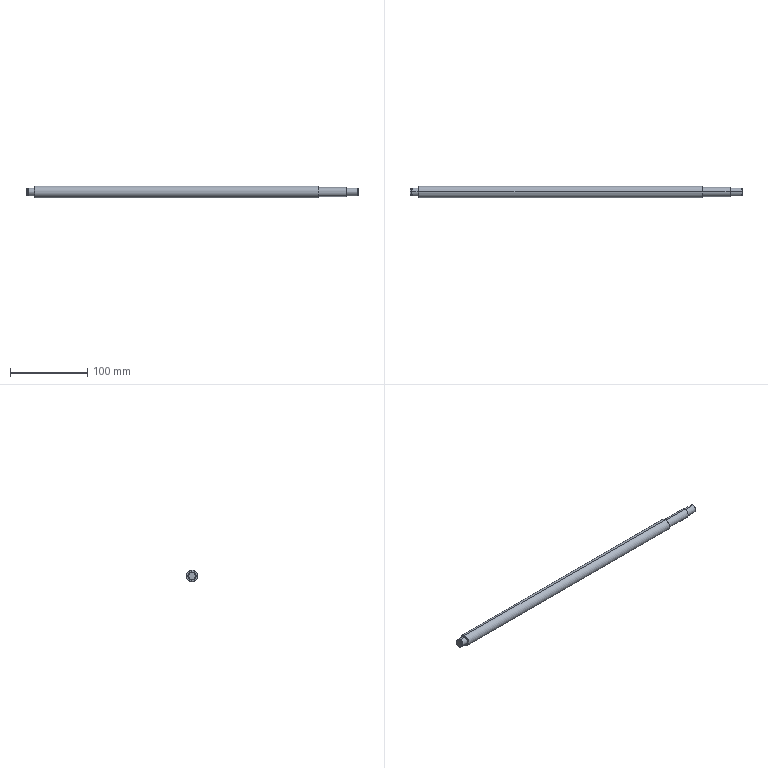Part | SolidWorks | features Revolution 8, RevCut 7, ICE 5, RefAxis 3, Fillet 2 | 1 solid | 35 faces | box 430 x 15 x 15 mm | volume 71115 mm3 | cylinder 12 | cone 10 | plane 7 | torus 6 | commonest cylinder face diameters 10 x6 9.6 x2 12 x2 15 x2
STEP:
#1=CARTESIAN_POINT('',(430.,0.,4.5));
#2=VERTEX_POINT('',#1);
#3=CARTESIAN_POINT('',(430.,0.,-4.5));
#4=VERTEX_POINT('',#3);
#5=CARTESIAN_POINT('',(430.,0.,0.));
#6=DIRECTION('',(-1.,0.,0.));
#7=DIRECTION('',(0.,0.,1.));
#8=AXIS2_PLACEMENT_3D('',#5,#6,#7);
#9=CIRCLE('',#8,4.5);
#10=EDGE_CURVE('',#2,#4,#9,.T.);
#11=ORIENTED_EDGE('',*,*,#10,.T.);
#12=CARTESIAN_POINT('',(429.5,0.,-5.));
#13=VERTEX_POINT('',#12);
#14=CARTESIAN_POINT('',(430.,0.,-4.5));
#15=DIRECTION('',(-0.7071,0.,-0.7071));
#16=VECTOR('',#15,1000.);
#17=LINE('',#14,#16);
#18=EDGE_CURVE('',#4,#13,#17,.T.);
#19=ORIENTED_EDGE('',*,*,#18,.T.);
#20=CARTESIAN_POINT('',(429.5,0.,5.));
#21=VERTEX_POINT('',#20);
#22=CARTESIAN_POINT('',(429.5,0.,0.));
#23=DIRECTION('',(-1.,0.,0.));
#24=DIRECTION('',(0.,0.,1.));
#25=AXIS2_PLACEMENT_3D('',#22,#23,#24);
#26=CIRCLE('',#25,5.);
#27=EDGE_CURVE('',#21,#13,#26,.T.);
#28=ORIENTED_EDGE('',*,*,#27,.F.);
#29=CARTESIAN_POINT('',(430.,0.,4.5));
#30=DIRECTION('',(-0.7071,0.,0.7071));
#31=VECTOR('',#30,1000.);
#32=LINE('',#29,#31);
#33=EDGE_CURVE('',#2,#21,#32,.T.);
#34=ORIENTED_EDGE('',*,*,#33,.F.);
#35=EDGE_LOOP('',(#11,#19,#28,#34));
#36=FACE_OUTER_BOUND('',#35,.T.);
#37=CARTESIAN_POINT('',(430.,0.,0.));
#38=DIRECTION('',(-1.,0.,0.));
#39=DIRECTION('',(0.,0.,1.));
#40=AXIS2_PLACEMENT_3D('',#37,#38,#39);
#41=CONICAL_SURFACE('',#40,4.5,0.7854);
#42=ADVANCED_FACE('',(#36),#41,.T.);
#43=ORIENTED_EDGE('',*,*,#27,.T.);
#44=CARTESIAN_POINT('',(415.2,0.,-5.));
#45=VERTEX_POINT('',#44);
#46=CARTESIAN_POINT('',(-7.5,0.,-5.));
#47=DIRECTION('',(-1.,0.,0.));
#48=VECTOR('',#47,1000.);
#49=LINE('',#46,#48);
#50=EDGE_CURVE('',#13,#45,#49,.T.);
#51=ORIENTED_EDGE('',*,*,#50,.T.);
#52=CARTESIAN_POINT('',(415.2,0.,5.));
#53=VERTEX_POINT('',#52);
#54=CARTESIAN_POINT('',(415.2,0.,0.));
#55=DIRECTION('',(-1.,0.,0.));
#56=DIRECTION('',(0.,0.,1.));
#57=AXIS2_PLACEMENT_3D('',#54,#55,#56);
#58=CIRCLE('',#57,5.);
#59=EDGE_CURVE('',#53,#45,#58,.T.);
#60=ORIENTED_EDGE('',*,*,#59,.F.);
#61=CARTESIAN_POINT('',(-7.5,0.,5.));
#62=DIRECTION('',(-1.,0.,0.));
#63=VECTOR('',#62,1000.);
#64=LINE('',#61,#63);
#65=EDGE_CURVE('',#21,#53,#64,.T.);
#66=ORIENTED_EDGE('',*,*,#65,.F.);
#67=EDGE_LOOP('',(#43,#51,#60,#66));
#68=FACE_OUTER_BOUND('',#67,.T.);
#69=CARTESIAN_POINT('',(-7.5,0.,0.));
#70=DIRECTION('',(-1.,0.,0.));
#71=DIRECTION('',(0.,0.,1.));
#72=AXIS2_PLACEMENT_3D('',#69,#70,#71);
#73=CYLINDRICAL_SURFACE('',#72,5.);
#74=ADVANCED_FACE('',(#68),#73,.T.);
#75=CARTESIAN_POINT('',(415.,0.,-5.2));
#76=VERTEX_POINT('',#75);
#77=CARTESIAN_POINT('',(415.,0.,5.2));
#78=VERTEX_POINT('',#77);
#79=CARTESIAN_POINT('',(415.,0.,0.));
#80=DIRECTION('',(-1.,0.,0.));
#81=DIRECTION('',(0.,0.,1.));
#82=AXIS2_PLACEMENT_3D('',#79,#80,#81);
#83=CIRCLE('',#82,5.2);
#84=EDGE_CURVE('',#76,#78,#83,.T.);
#85=ORIENTED_EDGE('',*,*,#84,.F.);
#86=CARTESIAN_POINT('',(415.2,0.,-5.2));
#87=DIRECTION('',(0.,1.,0.));
#88=DIRECTION('',(0.,0.,1.));
#89=AXIS2_PLACEMENT_3D('',#86,#87,#88);
#90=CIRCLE('',#89,0.2);
#91=EDGE_CURVE('',#76,#45,#90,.T.);
#92=ORIENTED_EDGE('',*,*,#91,.T.);
#93=CARTESIAN_POINT('',(415.2,0.,0.));
#94=DIRECTION('',(-1.,0.,0.));
#95=DIRECTION('',(0.,0.,1.));
#96=AXIS2_PLACEMENT_3D('',#93,#94,#95);
#97=CIRCLE('',#96,5.);
#98=EDGE_CURVE('',#45,#53,#97,.T.);
#99=ORIENTED_EDGE('',*,*,#98,.T.);
#100=CARTESIAN_POINT('',(415.2,0.,5.2));
#101=DIRECTION('',(0.,-1.,0.));
#102=DIRECTION('',(0.,0.,-1.));
#103=AXIS2_PLACEMENT_3D('',#100,#101,#102);
#104=CIRCLE('',#103,0.2);
#105=EDGE_CURVE('',#78,#53,#104,.T.);
#106=ORIENTED_EDGE('',*,*,#105,.F.);
#107=EDGE_LOOP('',(#85,#92,#99,#106));
#108=FACE_OUTER_BOUND('',#107,.T.);
#109=CARTESIAN_POINT('',(415.2,0.,0.));
#110=DIRECTION('',(-1.,0.,0.));
#111=DIRECTION('',(0.,0.,1.));
#112=AXIS2_PLACEMENT_3D('',#109,#110,#111);
#113=TOROIDAL_SURFACE('',#112,5.2,0.2);
#114=ADVANCED_FACE('',(#108),#113,.F.);
#115=CARTESIAN_POINT('',(415.,0.,5.5));
#116=VERTEX_POINT('',#115);
#117=CARTESIAN_POINT('',(415.,0.,-5.5));
#118=VERTEX_POINT('',#117);
#119=CARTESIAN_POINT('',(415.,0.,0.));
#120=DIRECTION('',(-1.,0.,0.));
#121=DIRECTION('',(0.,0.,1.));
#122=AXIS2_PLACEMENT_3D('',#119,#120,#121);
#123=CIRCLE('',#122,5.5);
#124=EDGE_CURVE('',#116,#118,#123,.T.);
#125=ORIENTED_EDGE('',*,*,#124,.T.);
#126=CARTESIAN_POINT('',(414.5,0.,-6.));
#127=VERTEX_POINT('',#126);
#128=CARTESIAN_POINT('',(415.,0.,-5.5));
#129=DIRECTION('',(-0.7071,0.,-0.7071));
#130=VECTOR('',#129,1000.);
#131=LINE('',#128,#130);
#132=EDGE_CURVE('',#118,#127,#131,.T.);
#133=ORIENTED_EDGE('',*,*,#132,.T.);
#134=CARTESIAN_POINT('',(414.5,0.,6.));
#135=VERTEX_POINT('',#134);
#136=CARTESIAN_POINT('',(414.5,0.,0.));
#137=DIRECTION('',(-1.,0.,0.));
#138=DIRECTION('',(0.,0.,1.));
#139=AXIS2_PLACEMENT_3D('',#136,#137,#138);
#140=CIRCLE('',#139,6.);
#141=EDGE_CURVE('',#135,#127,#140,.T.);
#142=ORIENTED_EDGE('',*,*,#141,.F.);
#143=CARTESIAN_POINT('',(415.,0.,5.5));
#144=DIRECTION('',(-0.7071,0.,0.7071));
#145=VECTOR('',#144,1000.);
#146=LINE('',#143,#145);
#147=EDGE_CURVE('',#116,#135,#146,.T.);
#148=ORIENTED_EDGE('',*,*,#147,.F.);
#149=EDGE_LOOP('',(#125,#133,#142,#148));
#150=FACE_OUTER_BOUND('',#149,.T.);
#151=CARTESIAN_POINT('',(415.,0.,0.));
#152=DIRECTION('',(-1.,0.,0.));
#153=DIRECTION('',(0.,0.,1.));
#154=AXIS2_PLACEMENT_3D('',#151,#152,#153);
#155=CONICAL_SURFACE('',#154,5.5,0.7854);
#156=ADVANCED_FACE('',(#150),#155,.T.);
#157=ORIENTED_EDGE('',*,*,#141,.T.);
#158=CARTESIAN_POINT('',(379.3,0.,-6.));
#159=VERTEX_POINT('',#158);
#160=CARTESIAN_POINT('',(-7.5,0.,-6.));
#161=DIRECTION('',(-1.,0.,0.));
#162=VECTOR('',#161,1000.);
#163=LINE('',#160,#162);
#164=EDGE_CURVE('',#127,#159,#163,.T.);
#165=ORIENTED_EDGE('',*,*,#164,.T.);
#166=CARTESIAN_POINT('',(379.3,0.,6.));
#167=VERTEX_POINT('',#166);
#168=CARTESIAN_POINT('',(379.3,0.,0.));
#169=DIRECTION('',(-1.,0.,0.));
#170=DIRECTION('',(0.,0.,1.));
#171=AXIS2_PLACEMENT_3D('',#168,#169,#170);
#172=CIRCLE('',#171,6.);
#173=EDGE_CURVE('',#167,#159,#172,.T.);
#174=ORIENTED_EDGE('',*,*,#173,.F.);
#175=CARTESIAN_POINT('',(-7.5,0.,6.));
#176=DIRECTION('',(-1.,0.,0.));
#177=VECTOR('',#176,1000.);
#178=LINE('',#175,#177);
#179=EDGE_CURVE('',#135,#167,#178,.T.);
#180=ORIENTED_EDGE('',*,*,#179,.F.);
#181=EDGE_LOOP('',(#157,#165,#174,#180));
#182=FACE_OUTER_BOUND('',#181,.T.);
#183=CARTESIAN_POINT('',(-7.5,0.,0.));
#184=DIRECTION('',(-1.,0.,0.));
#185=DIRECTION('',(0.,0.,1.));
#186=AXIS2_PLACEMENT_3D('',#183,#184,#185);
#187=CYLINDRICAL_SURFACE('',#186,6.);
#188=ADVANCED_FACE('',(#182),#187,.T.);
#189=CARTESIAN_POINT('',(379.,0.,-6.3));
#190=VERTEX_POINT('',#189);
#191=CARTESIAN_POINT('',(379.,0.,6.3));
#192=VERTEX_POINT('',#191);
#193=CARTESIAN_POINT('',(379.,0.,0.));
#194=DIRECTION('',(-1.,0.,0.));
#195=DIRECTION('',(0.,0.,1.));
#196=AXIS2_PLACEMENT_3D('',#193,#194,#195);
#197=CIRCLE('',#196,6.3);
#198=EDGE_CURVE('',#190,#192,#197,.T.);
#199=ORIENTED_EDGE('',*,*,#198,.F.);
#200=CARTESIAN_POINT('',(379.3,0.,-6.3));
#201=DIRECTION('',(0.,1.,0.));
#202=DIRECTION('',(0.,0.,1.));
#203=AXIS2_PLACEMENT_3D('',#200,#201,#202);
#204=CIRCLE('',#203,0.3);
#205=EDGE_CURVE('',#190,#159,#204,.T.);
#206=ORIENTED_EDGE('',*,*,#205,.T.);
#207=CARTESIAN_POINT('',(379.3,0.,0.));
#208=DIRECTION('',(-1.,0.,0.));
#209=DIRECTION('',(0.,0.,1.));
#210=AXIS2_PLACEMENT_3D('',#207,#208,#209);
#211=CIRCLE('',#210,6.);
#212=EDGE_CURVE('',#159,#167,#211,.T.);
#213=ORIENTED_EDGE('',*,*,#212,.T.);
#214=CARTESIAN_POINT('',(379.3,0.,6.3));
#215=DIRECTION('',(0.,-1.,0.));
#216=DIRECTION('',(0.,0.,-1.));
#217=AXIS2_PLACEMENT_3D('',#214,#215,#216);
#218=CIRCLE('',#217,0.3);
#219=EDGE_CURVE('',#192,#167,#218,.T.);
#220=ORIENTED_EDGE('',*,*,#219,.F.);
#221=EDGE_LOOP('',(#199,#206,#213,#220));
#222=FACE_OUTER_BOUND('',#221,.T.);
#223=CARTESIAN_POINT('',(379.3,0.,0.));
#224=DIRECTION('',(-1.,0.,0.));
#225=DIRECTION('',(0.,0.,1.));
#226=AXIS2_PLACEMENT_3D('',#223,#224,#225);
#227=TOROIDAL_SURFACE('',#226,6.3,0.3);
#228=ADVANCED_FACE('',(#222),#227,.F.);
#229=CARTESIAN_POINT('',(379.,0.,7.));
#230=VERTEX_POINT('',#229);
#231=CARTESIAN_POINT('',(379.,0.,-7.));
#232=VERTEX_POINT('',#231);
#233=CARTESIAN_POINT('',(379.,0.,0.));
#234=DIRECTION('',(-1.,0.,0.));
#235=DIRECTION('',(0.,0.,1.));
#236=AXIS2_PLACEMENT_3D('',#233,#234,#235);
#237=CIRCLE('',#236,7.);
#238=EDGE_CURVE('',#230,#232,#237,.T.);
#239=ORIENTED_EDGE('',*,*,#238,.T.);
#240=CARTESIAN_POINT('',(378.5,0.,-7.5));
#241=VERTEX_POINT('',#240);
#242=CARTESIAN_POINT('',(379.,0.,-7.));
#243=DIRECTION('',(-0.7071,0.,-0.7071));
#244=VECTOR('',#243,1000.);
#245=LINE('',#242,#244);
#246=EDGE_CURVE('',#232,#241,#245,.T.);
#247=ORIENTED_EDGE('',*,*,#246,.T.);
#248=CARTESIAN_POINT('',(378.5,0.,7.5));
#249=VERTEX_POINT('',#248);
#250=CARTESIAN_POINT('',(378.5,0.,0.));
#251=DIRECTION('',(-1.,0.,0.));
#252=DIRECTION('',(0.,0.,1.));
#253=AXIS2_PLACEMENT_3D('',#250,#251,#252);
#254=CIRCLE('',#253,7.5);
#255=EDGE_CURVE('',#249,#241,#254,.T.);
#256=ORIENTED_EDGE('',*,*,#255,.F.);
#257=CARTESIAN_POINT('',(379.,0.,7.));
#258=DIRECTION('',(-0.7071,0.,0.7071));
#259=VECTOR('',#258,1000.);
#260=LINE('',#257,#259);
#261=EDGE_CURVE('',#230,#249,#260,.T.);
#262=ORIENTED_EDGE('',*,*,#261,.F.);
#263=EDGE_LOOP('',(#239,#247,#256,#262));
#264=FACE_OUTER_BOUND('',#263,.T.);
#265=CARTESIAN_POINT('',(379.,0.,0.));
#266=DIRECTION('',(-1.,0.,0.));
#267=DIRECTION('',(0.,0.,1.));
#268=AXIS2_PLACEMENT_3D('',#265,#266,#267);
#269=CONICAL_SURFACE('',#268,7.,0.7854);
#270=ADVANCED_FACE('',(#264),#269,.T.);
#271=ORIENTED_EDGE('',*,*,#255,.T.);
#272=CARTESIAN_POINT('',(11.5,0.,-7.5));
#273=VERTEX_POINT('',#272);
#274=CARTESIAN_POINT('',(-7.5,0.,-7.5));
#275=DIRECTION('',(-1.,0.,0.));
#276=VECTOR('',#275,1000.);
#277=LINE('',#274,#276);
#278=EDGE_CURVE('',#241,#273,#277,.T.);
#279=ORIENTED_EDGE('',*,*,#278,.T.);
#280=CARTESIAN_POINT('',(11.5,0.,7.5));
#281=VERTEX_POINT('',#280);
#282=CARTESIAN_POINT('',(11.5,0.,0.));
#283=DIRECTION('',(-1.,0.,0.));
#284=DIRECTION('',(0.,0.,1.));
#285=AXIS2_PLACEMENT_3D('',#282,#283,#284);
#286=CIRCLE('',#285,7.5);
#287=EDGE_CURVE('',#281,#273,#286,.T.);
#288=ORIENTED_EDGE('',*,*,#287,.F.);
#289=CARTESIAN_POINT('',(-7.5,0.,7.5));
#290=DIRECTION('',(-1.,0.,0.));
#291=VECTOR('',#290,1000.);
#292=LINE('',#289,#291);
#293=EDGE_CURVE('',#249,#281,#292,.T.);
#294=ORIENTED_EDGE('',*,*,#293,.F.);
#295=EDGE_LOOP('',(#271,#279,#288,#294));
#296=FACE_OUTER_BOUND('',#295,.T.);
#297=CARTESIAN_POINT('',(-7.5,0.,0.));
#298=DIRECTION('',(-1.,0.,0.));
#299=DIRECTION('',(0.,0.,1.));
#300=AXIS2_PLACEMENT_3D('',#297,#298,#299);
#301=CYLINDRICAL_SURFACE('',#300,7.5);
#302=ADVANCED_FACE('',(#296),#301,.T.);
#303=CARTESIAN_POINT('',(11.,0.,7.));
#304=VERTEX_POINT('',#303);
#305=CARTESIAN_POINT('',(11.,0.,-7.));
#306=VERTEX_POINT('',#305);
#307=CARTESIAN_POINT('',(11.,0.,0.));
#308=DIRECTION('',(-1.,0.,0.));
#309=DIRECTION('',(0.,0.,1.));
#310=AXIS2_PLACEMENT_3D('',#307,#308,#309);
#311=CIRCLE('',#310,7.);
#312=EDGE_CURVE('',#304,#306,#311,.T.);
#313=ORIENTED_EDGE('',*,*,#312,.F.);
#314=CARTESIAN_POINT('',(11.5,0.,7.5));
#315=DIRECTION('',(0.7071,0.,0.7071));
#316=VECTOR('',#315,1000.);
#317=LINE('',#314,#316);
#318=EDGE_CURVE('',#304,#281,#317,.T.);
#319=ORIENTED_EDGE('',*,*,#318,.T.);
#320=ORIENTED_EDGE('',*,*,#287,.T.);
#321=CARTESIAN_POINT('',(11.5,0.,-7.5));
#322=DIRECTION('',(0.7071,0.,-0.7071));
#323=VECTOR('',#322,1000.);
#324=LINE('',#321,#323);
#325=EDGE_CURVE('',#306,#273,#324,.T.);
#326=ORIENTED_EDGE('',*,*,#325,.F.);
#327=EDGE_LOOP('',(#313,#319,#320,#326));
#328=FACE_OUTER_BOUND('',#327,.T.);
#329=CARTESIAN_POINT('',(11.5,0.,0.));
#330=DIRECTION('',(1.,0.,0.));
#331=DIRECTION('',(0.,0.,-1.));
#332=AXIS2_PLACEMENT_3D('',#329,#330,#331);
#333=CONICAL_SURFACE('',#332,7.5,0.7854);
#334=ADVANCED_FACE('',(#328),#333,.T.);
#335=CARTESIAN_POINT('',(10.7,0.,-5.));
#336=VERTEX_POINT('',#335);
#337=CARTESIAN_POINT('',(10.7,0.,5.));
#338=VERTEX_POINT('',#337);
#339=CARTESIAN_POINT('',(10.7,0.,0.));
#340=DIRECTION('',(-1.,0.,0.));
#341=DIRECTION('',(0.,0.,1.));
#342=AXIS2_PLACEMENT_3D('',#339,#340,#341);
#343=CIRCLE('',#342,5.);
#344=EDGE_CURVE('',#336,#338,#343,.T.);
#345=ORIENTED_EDGE('',*,*,#344,.F.);
#346=CARTESIAN_POINT('',(11.,0.,-5.3));
#347=VERTEX_POINT('',#346);
#348=CARTESIAN_POINT('',(10.7,0.,-5.3));
#349=DIRECTION('',(0.,1.,0.));
#350=DIRECTION('',(0.,0.,1.));
#351=AXIS2_PLACEMENT_3D('',#348,#349,#350);
#352=CIRCLE('',#351,0.3);
#353=EDGE_CURVE('',#336,#347,#352,.T.);
#354=ORIENTED_EDGE('',*,*,#353,.T.);
#355=CARTESIAN_POINT('',(11.,0.,5.3));
#356=VERTEX_POINT('',#355);
#357=CARTESIAN_POINT('',(11.,0.,0.));
#358=DIRECTION('',(-1.,0.,0.));
#359=DIRECTION('',(0.,0.,1.));
#360=AXIS2_PLACEMENT_3D('',#357,#358,#359);
#361=CIRCLE('',#360,5.3);
#362=EDGE_CURVE('',#347,#356,#361,.T.);
#363=ORIENTED_EDGE('',*,*,#362,.T.);
#364=CARTESIAN_POINT('',(10.7,0.,5.3));
#365=DIRECTION('',(0.,-1.,0.));
#366=DIRECTION('',(0.,0.,-1.));
#367=AXIS2_PLACEMENT_3D('',#364,#365,#366);
#368=CIRCLE('',#367,0.3);
#369=EDGE_CURVE('',#338,#356,#368,.T.);
#370=ORIENTED_EDGE('',*,*,#369,.F.);
#371=EDGE_LOOP('',(#345,#354,#363,#370));
#372=FACE_OUTER_BOUND('',#371,.T.);
#373=CARTESIAN_POINT('',(10.7,0.,0.));
#374=DIRECTION('',(-1.,0.,0.));
#375=DIRECTION('',(0.,0.,1.));
#376=AXIS2_PLACEMENT_3D('',#373,#374,#375);
#377=TOROIDAL_SURFACE('',#376,5.3,0.3);
#378=ADVANCED_FACE('',(#372),#377,.F.);
#379=CARTESIAN_POINT('',(10.7,0.,0.));
#380=DIRECTION('',(-1.,0.,0.));
#381=DIRECTION('',(0.,0.,1.));
#382=AXIS2_PLACEMENT_3D('',#379,#380,#381);
#383=CIRCLE('',#382,5.);
#384=EDGE_CURVE('',#338,#336,#383,.T.);
#385=ORIENTED_EDGE('',*,*,#384,.T.);
#386=CARTESIAN_POINT('',(3.,0.,-5.));
#387=VERTEX_POINT('',#386);
#388=CARTESIAN_POINT('',(-7.5,0.,-5.));
#389=DIRECTION('',(-1.,0.,0.));
#390=VECTOR('',#389,1000.);
#391=LINE('',#388,#390);
#392=EDGE_CURVE('',#336,#387,#391,.T.);
#393=ORIENTED_EDGE('',*,*,#392,.T.);
#394=CARTESIAN_POINT('',(3.,0.,5.));
#395=VERTEX_POINT('',#394);
#396=CARTESIAN_POINT('',(3.,0.,0.));
#397=DIRECTION('',(-1.,0.,0.));
#398=DIRECTION('',(0.,0.,1.));
#399=AXIS2_PLACEMENT_3D('',#396,#397,#398);
#400=CIRCLE('',#399,5.);
#401=EDGE_CURVE('',#395,#387,#400,.T.);
#402=ORIENTED_EDGE('',*,*,#401,.F.);
#403=CARTESIAN_POINT('',(-7.5,0.,5.));
#404=DIRECTION('',(-1.,0.,0.));
#405=VECTOR('',#404,1000.);
#406=LINE('',#403,#405);
#407=EDGE_CURVE('',#338,#395,#406,.T.);
#408=ORIENTED_EDGE('',*,*,#407,.F.);
#409=EDGE_LOOP('',(#385,#393,#402,#408));
#410=FACE_OUTER_BOUND('',#409,.T.);
#411=CARTESIAN_POINT('',(-7.5,0.,0.));
#412=DIRECTION('',(-1.,0.,0.));
#413=DIRECTION('',(0.,0.,1.));
#414=AXIS2_PLACEMENT_3D('',#411,#412,#413);
#415=CYLINDRICAL_SURFACE('',#414,5.);
#416=ADVANCED_FACE('',(#410),#415,.T.);
#417=CARTESIAN_POINT('',(3.,0.,4.8));
#418=VERTEX_POINT('',#417);
#419=CARTESIAN_POINT('',(3.,0.,-4.8));
#420=VERTEX_POINT('',#419);
#421=CARTESIAN_POINT('',(3.,0.,0.));
#422=DIRECTION('',(-1.,0.,0.));
#423=DIRECTION('',(0.,0.,1.));
#424=AXIS2_PLACEMENT_3D('',#421,#422,#423);
#425=CIRCLE('',#424,4.8);
#426=EDGE_CURVE('',#418,#420,#425,.T.);
#427=ORIENTED_EDGE('',*,*,#426,.T.);
#428=CARTESIAN_POINT('',(1.85,0.,-4.8));
#429=VERTEX_POINT('',#428);
#430=CARTESIAN_POINT('',(-7.5,0.,-4.8));
#431=DIRECTION('',(-1.,0.,0.));
#432=VECTOR('',#431,1000.);
#433=LINE('',#430,#432);
#434=EDGE_CURVE('',#420,#429,#433,.T.);
#435=ORIENTED_EDGE('',*,*,#434,.T.);
#436=CARTESIAN_POINT('',(1.85,0.,4.8));
#437=VERTEX_POINT('',#436);
#438=CARTESIAN_POINT('',(1.85,0.,0.));
#439=DIRECTION('',(-1.,0.,0.));
#440=DIRECTION('',(0.,0.,1.));
#441=AXIS2_PLACEMENT_3D('',#438,#439,#440);
#442=CIRCLE('',#441,4.8);
#443=EDGE_CURVE('',#437,#429,#442,.T.);
#444=ORIENTED_EDGE('',*,*,#443,.F.);
#445=CARTESIAN_POINT('',(-7.5,0.,4.8));
#446=DIRECTION('',(-1.,0.,0.));
#447=VECTOR('',#446,1000.);
#448=LINE('',#445,#447);
#449=EDGE_CURVE('',#418,#437,#448,.T.);
#450=ORIENTED_EDGE('',*,*,#449,.F.);
#451=EDGE_LOOP('',(#427,#435,#444,#450));
#452=FACE_OUTER_BOUND('',#451,.T.);
#453=CARTESIAN_POINT('',(-7.5,0.,0.));
#454=DIRECTION('',(-1.,0.,0.));
#455=DIRECTION('',(0.,0.,1.));
#456=AXIS2_PLACEMENT_3D('',#453,#454,#455);
#457=CYLINDRICAL_SURFACE('',#456,4.8);
#458=ADVANCED_FACE('',(#452),#457,.T.);
#459=CARTESIAN_POINT('',(1.85,0.,5.));
#460=VERTEX_POINT('',#459);
#461=CARTESIAN_POINT('',(1.85,0.,-5.));
#462=VERTEX_POINT('',#461);
#463=CARTESIAN_POINT('',(1.85,0.,0.));
#464=DIRECTION('',(-1.,0.,0.));
#465=DIRECTION('',(0.,0.,1.));
#466=AXIS2_PLACEMENT_3D('',#463,#464,#465);
#467=CIRCLE('',#466,5.);
#468=EDGE_CURVE('',#460,#462,#467,.T.);
#469=ORIENTED_EDGE('',*,*,#468,.T.);
#470=CARTESIAN_POINT('',(0.5,0.,-5.));
#471=VERTEX_POINT('',#470);
#472=CARTESIAN_POINT('',(-7.5,0.,-5.));
#473=DIRECTION('',(-1.,0.,0.));
#474=VECTOR('',#473,1000.);
#475=LINE('',#472,#474);
#476=EDGE_CURVE('',#462,#471,#475,.T.);
#477=ORIENTED_EDGE('',*,*,#476,.T.);
#478=CARTESIAN_POINT('',(0.5,0.,5.));
#479=VERTEX_POINT('',#478);
#480=CARTESIAN_POINT('',(0.5,0.,0.));
#481=DIRECTION('',(-1.,0.,0.));
#482=DIRECTION('',(0.,0.,1.));
#483=AXIS2_PLACEMENT_3D('',#480,#481,#482);
#484=CIRCLE('',#483,5.);
#485=EDGE_CURVE('',#479,#471,#484,.T.);
#486=ORIENTED_EDGE('',*,*,#485,.F.);
#487=CARTESIAN_POINT('',(-7.5,0.,5.));
#488=DIRECTION('',(-1.,0.,0.));
#489=VECTOR('',#488,1000.);
#490=LINE('',#487,#489);
#491=EDGE_CURVE('',#460,#479,#490,.T.);
#492=ORIENTED_EDGE('',*,*,#491,.F.);
#493=EDGE_LOOP('',(#469,#477,#486,#492));
#494=FACE_OUTER_BOUND('',#493,.T.);
#495=CARTESIAN_POINT('',(-7.5,0.,0.));
#496=DIRECTION('',(-1.,0.,0.));
#497=DIRECTION('',(0.,0.,1.));
#498=AXIS2_PLACEMENT_3D('',#495,#496,#497);
#499=CYLINDRICAL_SURFACE('',#498,5.);
#500=ADVANCED_FACE('',(#494),#499,.T.);
#501=CARTESIAN_POINT('',(0.,0.,4.5));
#502=VERTEX_POINT('',#501);
#503=CARTESIAN_POINT('',(0.,0.,-4.5));
#504=VERTEX_POINT('',#503);
#505=CARTESIAN_POINT('',(0.,0.,0.));
#506=DIRECTION('',(-1.,0.,0.));
#507=DIRECTION('',(0.,0.,1.));
#508=AXIS2_PLACEMENT_3D('',#505,#506,#507);
#509=CIRCLE('',#508,4.5);
#510=EDGE_CURVE('',#502,#504,#509,.T.);
#511=ORIENTED_EDGE('',*,*,#510,.F.);
#512=CARTESIAN_POINT('',(0.5,0.,5.));
#513=DIRECTION('',(0.7071,0.,0.7071));
#514=VECTOR('',#513,1000.);
#515=LINE('',#512,#514);
#516=EDGE_CURVE('',#502,#479,#515,.T.);
#517=ORIENTED_EDGE('',*,*,#516,.T.);
#518=ORIENTED_EDGE('',*,*,#485,.T.);
#519=CARTESIAN_POINT('',(0.5,0.,-5.));
#520=DIRECTION('',(0.7071,0.,-0.7071));
#521=VECTOR('',#520,1000.);
#522=LINE('',#519,#521);
#523=EDGE_CURVE('',#504,#471,#522,.T.);
#524=ORIENTED_EDGE('',*,*,#523,.F.);
#525=EDGE_LOOP('',(#511,#517,#518,#524));
#526=FACE_OUTER_BOUND('',#525,.T.);
#527=CARTESIAN_POINT('',(0.5,0.,0.));
#528=DIRECTION('',(1.,0.,0.));
#529=DIRECTION('',(0.,0.,-1.));
#530=AXIS2_PLACEMENT_3D('',#527,#528,#529);
#531=CONICAL_SURFACE('',#530,5.,0.7854);
#532=ADVANCED_FACE('',(#526),#531,.T.);
#533=ORIENTED_EDGE('',*,*,#516,.F.);
#534=CARTESIAN_POINT('',(0.,0.,0.));
#535=DIRECTION('',(-1.,0.,0.));
#536=DIRECTION('',(0.,0.,1.));
#537=AXIS2_PLACEMENT_3D('',#534,#535,#536);
#538=CIRCLE('',#537,4.5);
#539=EDGE_CURVE('',#504,#502,#538,.T.);
#540=ORIENTED_EDGE('',*,*,#539,.F.);
#541=ORIENTED_EDGE('',*,*,#523,.T.);
#542=CARTESIAN_POINT('',(0.5,0.,0.));
#543=DIRECTION('',(-1.,0.,0.));
#544=DIRECTION('',(0.,0.,1.));
#545=AXIS2_PLACEMENT_3D('',#542,#543,#544);
#546=CIRCLE('',#545,5.);
#547=EDGE_CURVE('',#471,#479,#546,.T.);
#548=ORIENTED_EDGE('',*,*,#547,.T.);
#549=EDGE_LOOP('',(#533,#540,#541,#548));
#550=FACE_OUTER_BOUND('',#549,.T.);
#551=CARTESIAN_POINT('',(0.5,0.,0.));
#552=DIRECTION('',(1.,0.,0.));
#553=DIRECTION('',(0.,0.,-1.));
#554=AXIS2_PLACEMENT_3D('',#551,#552,#553);
#555=CONICAL_SURFACE('',#554,5.,0.7854);
#556=ADVANCED_FACE('',(#550),#555,.T.);
#557=ORIENTED_EDGE('',*,*,#476,.F.);
#558=CARTESIAN_POINT('',(1.85,0.,0.));
#559=DIRECTION('',(-1.,0.,0.));
#560=DIRECTION('',(0.,0.,1.));
#561=AXIS2_PLACEMENT_3D('',#558,#559,#560);
#562=CIRCLE('',#561,5.);
#563=EDGE_CURVE('',#462,#460,#562,.T.);
#564=ORIENTED_EDGE('',*,*,#563,.T.);
#565=ORIENTED_EDGE('',*,*,#491,.T.);
#566=ORIENTED_EDGE('',*,*,#547,.F.);
#567=EDGE_LOOP('',(#557,#564,#565,#566));
#568=FACE_OUTER_BOUND('',#567,.T.);
#569=CARTESIAN_POINT('',(-7.5,0.,0.));
#570=DIRECTION('',(-1.,0.,0.));
#571=DIRECTION('',(0.,0.,1.));
#572=AXIS2_PLACEMENT_3D('',#569,#570,#571);
#573=CYLINDRICAL_SURFACE('',#572,5.);
#574=ADVANCED_FACE('',(#568),#573,.T.);
#575=ORIENTED_EDGE('',*,*,#468,.F.);
#576=ORIENTED_EDGE('',*,*,#563,.F.);
#577=EDGE_LOOP('',(#575,#576));
#578=FACE_OUTER_BOUND('',#577,.T.);
#579=ORIENTED_EDGE('',*,*,#443,.T.);
#580=CARTESIAN_POINT('',(1.85,0.,0.));
#581=DIRECTION('',(-1.,0.,0.));
#582=DIRECTION('',(0.,0.,1.));
#583=AXIS2_PLACEMENT_3D('',#580,#581,#582);
#584=CIRCLE('',#583,4.8);
#585=EDGE_CURVE('',#429,#437,#584,.T.);
#586=ORIENTED_EDGE('',*,*,#585,.T.);
#587=EDGE_LOOP('',(#579,#586));
#588=FACE_BOUND('',#587,.T.);
#589=CARTESIAN_POINT('',(1.85,5.,0.));
#590=DIRECTION('',(-1.,0.,0.));
#591=DIRECTION('',(0.,0.,1.));
#592=AXIS2_PLACEMENT_3D('',#589,#590,#591);
#593=PLANE('',#592);
#594=ADVANCED_FACE('',(#578,#588),#593,.F.);
#595=ORIENTED_EDGE('',*,*,#434,.F.);
#596=CARTESIAN_POINT('',(3.,0.,0.));
#597=DIRECTION('',(-1.,0.,0.));
#598=DIRECTION('',(0.,0.,1.));
#599=AXIS2_PLACEMENT_3D('',#596,#597,#598);
#600=CIRCLE('',#599,4.8);
#601=EDGE_CURVE('',#420,#418,#600,.T.);
#602=ORIENTED_EDGE('',*,*,#601,.T.);
#603=ORIENTED_EDGE('',*,*,#449,.T.);
#604=ORIENTED_EDGE('',*,*,#585,.F.);
#605=EDGE_LOOP('',(#595,#602,#603,#604));
#606=FACE_OUTER_BOUND('',#605,.T.);
#607=CARTESIAN_POINT('',(-7.5,0.,0.));
#608=DIRECTION('',(-1.,0.,0.));
#609=DIRECTION('',(0.,0.,1.));
#610=AXIS2_PLACEMENT_3D('',#607,#608,#609);
#611=CYLINDRICAL_SURFACE('',#610,4.8);
#612=ADVANCED_FACE('',(#606),#611,.T.);
#613=ORIENTED_EDGE('',*,*,#426,.F.);
#614=ORIENTED_EDGE('',*,*,#601,.F.);
#615=EDGE_LOOP('',(#613,#614));
#616=FACE_BOUND('',#615,.T.);
#617=ORIENTED_EDGE('',*,*,#401,.T.);
#618=CARTESIAN_POINT('',(3.,0.,0.));
#619=DIRECTION('',(-1.,0.,0.));
#620=DIRECTION('',(0.,0.,1.));
#621=AXIS2_PLACEMENT_3D('',#618,#619,#620);
#622=CIRCLE('',#621,5.);
#623=EDGE_CURVE('',#387,#395,#622,.T.);
#624=ORIENTED_EDGE('',*,*,#623,.T.);
#625=EDGE_LOOP('',(#617,#624));
#626=FACE_OUTER_BOUND('',#625,.T.);
#627=CARTESIAN_POINT('',(3.,5.,0.));
#628=DIRECTION('',(1.,0.,0.));
#629=DIRECTION('',(0.,0.,-1.));
#630=AXIS2_PLACEMENT_3D('',#627,#628,#629);
#631=PLANE('',#630);
#632=ADVANCED_FACE('',(#616,#626),#631,.F.);
#633=ORIENTED_EDGE('',*,*,#392,.F.);
#634=ORIENTED_EDGE('',*,*,#344,.T.);
#635=ORIENTED_EDGE('',*,*,#407,.T.);
#636=ORIENTED_EDGE('',*,*,#623,.F.);
#637=EDGE_LOOP('',(#633,#634,#635,#636));
#638=FACE_OUTER_BOUND('',#637,.T.);
#639=CARTESIAN_POINT('',(-7.5,0.,0.));
#640=DIRECTION('',(-1.,0.,0.));
#641=DIRECTION('',(0.,0.,1.));
#642=AXIS2_PLACEMENT_3D('',#639,#640,#641);
#643=CYLINDRICAL_SURFACE('',#642,5.);
#644=ADVANCED_FACE('',(#638),#643,.T.);
#645=ORIENTED_EDGE('',*,*,#353,.F.);
#646=ORIENTED_EDGE('',*,*,#384,.F.);
#647=ORIENTED_EDGE('',*,*,#369,.T.);
#648=CARTESIAN_POINT('',(11.,0.,0.));
#649=DIRECTION('',(-1.,0.,0.));
#650=DIRECTION('',(0.,0.,1.));
#651=AXIS2_PLACEMENT_3D('',#648,#649,#650);
#652=CIRCLE('',#651,5.3);
#653=EDGE_CURVE('',#356,#347,#652,.T.);
#654=ORIENTED_EDGE('',*,*,#653,.T.);
#655=EDGE_LOOP('',(#645,#646,#647,#654));
#656=FACE_OUTER_BOUND('',#655,.T.);
#657=CARTESIAN_POINT('',(10.7,0.,0.));
#658=DIRECTION('',(-1.,0.,0.));
#659=DIRECTION('',(0.,0.,1.));
#660=AXIS2_PLACEMENT_3D('',#657,#658,#659);
#661=TOROIDAL_SURFACE('',#660,5.3,0.3);
#662=ADVANCED_FACE('',(#656),#661,.F.);
#663=ORIENTED_EDGE('',*,*,#653,.F.);
#664=ORIENTED_EDGE('',*,*,#362,.F.);
#665=EDGE_LOOP('',(#663,#664));
#666=FACE_BOUND('',#665,.T.);
#667=CARTESIAN_POINT('',(11.,0.,0.));
#668=DIRECTION('',(-1.,0.,0.));
#669=DIRECTION('',(0.,0.,1.));
#670=AXIS2_PLACEMENT_3D('',#667,#668,#669);
#671=CIRCLE('',#670,7.);
#672=EDGE_CURVE('',#306,#304,#671,.T.);
#673=ORIENTED_EDGE('',*,*,#672,.T.);
#674=ORIENTED_EDGE('',*,*,#312,.T.);
#675=EDGE_LOOP('',(#673,#674));
#676=FACE_OUTER_BOUND('',#675,.T.);
#677=CARTESIAN_POINT('',(11.,7.,0.));
#678=DIRECTION('',(1.,0.,0.));
#679=DIRECTION('',(0.,0.,-1.));
#680=AXIS2_PLACEMENT_3D('',#677,#678,#679);
#681=PLANE('',#680);
#682=ADVANCED_FACE('',(#666,#676),#681,.F.);
#683=ORIENTED_EDGE('',*,*,#318,.F.);
#684=ORIENTED_EDGE('',*,*,#672,.F.);
#685=ORIENTED_EDGE('',*,*,#325,.T.);
#686=CARTESIAN_POINT('',(11.5,0.,0.));
#687=DIRECTION('',(-1.,0.,0.));
#688=DIRECTION('',(0.,0.,1.));
#689=AXIS2_PLACEMENT_3D('',#686,#687,#688);
#690=CIRCLE('',#689,7.5);
#691=EDGE_CURVE('',#273,#281,#690,.T.);
#692=ORIENTED_EDGE('',*,*,#691,.T.);
#693=EDGE_LOOP('',(#683,#684,#685,#692));
#694=FACE_OUTER_BOUND('',#693,.T.);
#695=CARTESIAN_POINT('',(11.5,0.,0.));
#696=DIRECTION('',(1.,0.,0.));
#697=DIRECTION('',(0.,0.,-1.));
#698=AXIS2_PLACEMENT_3D('',#695,#696,#697);
#699=CONICAL_SURFACE('',#698,7.5,0.7854);
#700=ADVANCED_FACE('',(#694),#699,.T.);
#701=ORIENTED_EDGE('',*,*,#278,.F.);
#702=CARTESIAN_POINT('',(378.5,0.,0.));
#703=DIRECTION('',(-1.,0.,0.));
#704=DIRECTION('',(0.,0.,1.));
#705=AXIS2_PLACEMENT_3D('',#702,#703,#704);
#706=CIRCLE('',#705,7.5);
#707=EDGE_CURVE('',#241,#249,#706,.T.);
#708=ORIENTED_EDGE('',*,*,#707,.T.);
#709=ORIENTED_EDGE('',*,*,#293,.T.);
#710=ORIENTED_EDGE('',*,*,#691,.F.);
#711=EDGE_LOOP('',(#701,#708,#709,#710));
#712=FACE_OUTER_BOUND('',#711,.T.);
#713=CARTESIAN_POINT('',(-7.5,0.,0.));
#714=DIRECTION('',(-1.,0.,0.));
#715=DIRECTION('',(0.,0.,1.));
#716=AXIS2_PLACEMENT_3D('',#713,#714,#715);
#717=CYLINDRICAL_SURFACE('',#716,7.5);
#718=ADVANCED_FACE('',(#712),#717,.T.);
#719=ORIENTED_EDGE('',*,*,#246,.F.);
#720=CARTESIAN_POINT('',(379.,0.,0.));
#721=DIRECTION('',(-1.,0.,0.));
#722=DIRECTION('',(0.,0.,1.));
#723=AXIS2_PLACEMENT_3D('',#720,#721,#722);
#724=CIRCLE('',#723,7.);
#725=EDGE_CURVE('',#232,#230,#724,.T.);
#726=ORIENTED_EDGE('',*,*,#725,.T.);
#727=ORIENTED_EDGE('',*,*,#261,.T.);
#728=ORIENTED_EDGE('',*,*,#707,.F.);
#729=EDGE_LOOP('',(#719,#726,#727,#728));
#730=FACE_OUTER_BOUND('',#729,.T.);
#731=CARTESIAN_POINT('',(379.,0.,0.));
#732=DIRECTION('',(-1.,0.,0.));
#733=DIRECTION('',(0.,0.,1.));
#734=AXIS2_PLACEMENT_3D('',#731,#732,#733);
#735=CONICAL_SURFACE('',#734,7.,0.7854);
#736=ADVANCED_FACE('',(#730),#735,.T.);
#737=ORIENTED_EDGE('',*,*,#238,.F.);
#738=ORIENTED_EDGE('',*,*,#725,.F.);
#739=EDGE_LOOP('',(#737,#738));
#740=FACE_OUTER_BOUND('',#739,.T.);
#741=CARTESIAN_POINT('',(379.,0.,0.));
#742=DIRECTION('',(-1.,0.,0.));
#743=DIRECTION('',(0.,0.,1.));
#744=AXIS2_PLACEMENT_3D('',#741,#742,#743);
#745=CIRCLE('',#744,6.3);
#746=EDGE_CURVE('',#192,#190,#745,.T.);
#747=ORIENTED_EDGE('',*,*,#746,.T.);
#748=ORIENTED_EDGE('',*,*,#198,.T.);
#749=EDGE_LOOP('',(#747,#748));
#750=FACE_BOUND('',#749,.T.);
#751=CARTESIAN_POINT('',(379.,6.3,0.));
#752=DIRECTION('',(-1.,0.,0.));
#753=DIRECTION('',(0.,0.,1.));
#754=AXIS2_PLACEMENT_3D('',#751,#752,#753);
#755=PLANE('',#754);
#756=ADVANCED_FACE('',(#740,#750),#755,.F.);
#757=ORIENTED_EDGE('',*,*,#205,.F.);
#758=ORIENTED_EDGE('',*,*,#746,.F.);
#759=ORIENTED_EDGE('',*,*,#219,.T.);
#760=ORIENTED_EDGE('',*,*,#173,.T.);
#761=EDGE_LOOP('',(#757,#758,#759,#760));
#762=FACE_OUTER_BOUND('',#761,.T.);
#763=CARTESIAN_POINT('',(379.3,0.,0.));
#764=DIRECTION('',(-1.,0.,0.));
#765=DIRECTION('',(0.,0.,1.));
#766=AXIS2_PLACEMENT_3D('',#763,#764,#765);
#767=TOROIDAL_SURFACE('',#766,6.3,0.3);
#768=ADVANCED_FACE('',(#762),#767,.F.);
#769=ORIENTED_EDGE('',*,*,#164,.F.);
#770=CARTESIAN_POINT('',(414.5,0.,0.));
#771=DIRECTION('',(-1.,0.,0.));
#772=DIRECTION('',(0.,0.,1.));
#773=AXIS2_PLACEMENT_3D('',#770,#771,#772);
#774=CIRCLE('',#773,6.);
#775=EDGE_CURVE('',#127,#135,#774,.T.);
#776=ORIENTED_EDGE('',*,*,#775,.T.);
#777=ORIENTED_EDGE('',*,*,#179,.T.);
#778=ORIENTED_EDGE('',*,*,#212,.F.);
#779=EDGE_LOOP('',(#769,#776,#777,#778));
#780=FACE_OUTER_BOUND('',#779,.T.);
#781=CARTESIAN_POINT('',(-7.5,0.,0.));
#782=DIRECTION('',(-1.,0.,0.));
#783=DIRECTION('',(0.,0.,1.));
#784=AXIS2_PLACEMENT_3D('',#781,#782,#783);
#785=CYLINDRICAL_SURFACE('',#784,6.);
#786=ADVANCED_FACE('',(#780),#785,.T.);
#787=ORIENTED_EDGE('',*,*,#132,.F.);
#788=CARTESIAN_POINT('',(415.,0.,0.));
#789=DIRECTION('',(-1.,0.,0.));
#790=DIRECTION('',(0.,0.,1.));
#791=AXIS2_PLACEMENT_3D('',#788,#789,#790);
#792=CIRCLE('',#791,5.5);
#793=EDGE_CURVE('',#118,#116,#792,.T.);
#794=ORIENTED_EDGE('',*,*,#793,.T.);
#795=ORIENTED_EDGE('',*,*,#147,.T.);
#796=ORIENTED_EDGE('',*,*,#775,.F.);
#797=EDGE_LOOP('',(#787,#794,#795,#796));
#798=FACE_OUTER_BOUND('',#797,.T.);
#799=CARTESIAN_POINT('',(415.,0.,0.));
#800=DIRECTION('',(-1.,0.,0.));
#801=DIRECTION('',(0.,0.,1.));
#802=AXIS2_PLACEMENT_3D('',#799,#800,#801);
#803=CONICAL_SURFACE('',#802,5.5,0.7854);
#804=ADVANCED_FACE('',(#798),#803,.T.);
#805=ORIENTED_EDGE('',*,*,#124,.F.);
#806=ORIENTED_EDGE('',*,*,#793,.F.);
#807=EDGE_LOOP('',(#805,#806));
#808=FACE_OUTER_BOUND('',#807,.T.);
#809=CARTESIAN_POINT('',(415.,0.,0.));
#810=DIRECTION('',(-1.,0.,0.));
#811=DIRECTION('',(0.,0.,1.));
#812=AXIS2_PLACEMENT_3D('',#809,#810,#811);
#813=CIRCLE('',#812,5.2);
#814=EDGE_CURVE('',#78,#76,#813,.T.);
#815=ORIENTED_EDGE('',*,*,#814,.T.);
#816=ORIENTED_EDGE('',*,*,#84,.T.);
#817=EDGE_LOOP('',(#815,#816));
#818=FACE_BOUND('',#817,.T.);
#819=CARTESIAN_POINT('',(415.,5.2,0.));
#820=DIRECTION('',(-1.,0.,0.));
#821=DIRECTION('',(0.,0.,1.));
#822=AXIS2_PLACEMENT_3D('',#819,#820,#821);
#823=PLANE('',#822);
#824=ADVANCED_FACE('',(#808,#818),#823,.F.);
#825=ORIENTED_EDGE('',*,*,#91,.F.);
#826=ORIENTED_EDGE('',*,*,#814,.F.);
#827=ORIENTED_EDGE('',*,*,#105,.T.);
#828=ORIENTED_EDGE('',*,*,#59,.T.);
#829=EDGE_LOOP('',(#825,#826,#827,#828));
#830=FACE_OUTER_BOUND('',#829,.T.);
#831=CARTESIAN_POINT('',(415.2,0.,0.));
#832=DIRECTION('',(-1.,0.,0.));
#833=DIRECTION('',(0.,0.,1.));
#834=AXIS2_PLACEMENT_3D('',#831,#832,#833);
#835=TOROIDAL_SURFACE('',#834,5.2,0.2);
#836=ADVANCED_FACE('',(#830),#835,.F.);
#837=ORIENTED_EDGE('',*,*,#50,.F.);
#838=CARTESIAN_POINT('',(429.5,0.,0.));
#839=DIRECTION('',(-1.,0.,0.));
#840=DIRECTION('',(0.,0.,1.));
#841=AXIS2_PLACEMENT_3D('',#838,#839,#840);
#842=CIRCLE('',#841,5.);
#843=EDGE_CURVE('',#13,#21,#842,.T.);
#844=ORIENTED_EDGE('',*,*,#843,.T.);
#845=ORIENTED_EDGE('',*,*,#65,.T.);
#846=ORIENTED_EDGE('',*,*,#98,.F.);
#847=EDGE_LOOP('',(#837,#844,#845,#846));
#848=FACE_OUTER_BOUND('',#847,.T.);
#849=CARTESIAN_POINT('',(-7.5,0.,0.));
#850=DIRECTION('',(-1.,0.,0.));
#851=DIRECTION('',(0.,0.,1.));
#852=AXIS2_PLACEMENT_3D('',#849,#850,#851);
#853=CYLINDRICAL_SURFACE('',#852,5.);
#854=ADVANCED_FACE('',(#848),#853,.T.);
#855=ORIENTED_EDGE('',*,*,#18,.F.);
#856=CARTESIAN_POINT('',(430.,0.,0.));
#857=DIRECTION('',(-1.,0.,0.));
#858=DIRECTION('',(0.,0.,1.));
#859=AXIS2_PLACEMENT_3D('',#856,#857,#858);
#860=CIRCLE('',#859,4.5);
#861=EDGE_CURVE('',#4,#2,#860,.T.);
#862=ORIENTED_EDGE('',*,*,#861,.T.);
#863=ORIENTED_EDGE('',*,*,#33,.T.);
#864=ORIENTED_EDGE('',*,*,#843,.F.);
#865=EDGE_LOOP('',(#855,#862,#863,#864));
#866=FACE_OUTER_BOUND('',#865,.T.);
#867=CARTESIAN_POINT('',(430.,0.,0.));
#868=DIRECTION('',(-1.,0.,0.));
#869=DIRECTION('',(0.,0.,1.));
#870=AXIS2_PLACEMENT_3D('',#867,#868,#869);
#871=CONICAL_SURFACE('',#870,4.5,0.7854);
#872=ADVANCED_FACE('',(#866),#871,.T.);
#873=ORIENTED_EDGE('',*,*,#10,.F.);
#874=ORIENTED_EDGE('',*,*,#861,.F.);
#875=EDGE_LOOP('',(#873,#874));
#876=FACE_OUTER_BOUND('',#875,.T.);
#877=CARTESIAN_POINT('',(430.,0.,0.));
#878=DIRECTION('',(-1.,0.,0.));
#879=DIRECTION('',(0.,0.,1.));
#880=AXIS2_PLACEMENT_3D('',#877,#878,#879);
#881=PLANE('',#880);
#882=ADVANCED_FACE('',(#876),#881,.F.);
#883=ORIENTED_EDGE('',*,*,#539,.T.);
#884=ORIENTED_EDGE('',*,*,#510,.T.);
#885=EDGE_LOOP('',(#883,#884));
#886=FACE_OUTER_BOUND('',#885,.T.);
#887=CARTESIAN_POINT('',(0.,4.5,0.));
#888=DIRECTION('',(1.,0.,0.));
#889=DIRECTION('',(0.,0.,-1.));
#890=AXIS2_PLACEMENT_3D('',#887,#888,#889);
#891=PLANE('',#890);
#892=ADVANCED_FACE('',(#886),#891,.F.);
#893=CLOSED_SHELL('',(#42,#74,#114,#156,#188,#228,#270,#302,#334,#378,#416,#458,#500,#532,#556,#574,#594,#612,#632,#644,#662,#682,#700,#718,#736,#756,#768,#786,#804,#824,#836,#854,#872,#882,#892));
#894=MANIFOLD_SOLID_BREP('',#893);
#895=CARTESIAN_POINT('',(0.,0.,0.));
#896=DIRECTION('',(0.,0.,1.));
#897=DIRECTION('',(1.,0.,0.));
#898=AXIS2_PLACEMENT_3D('',#895,#896,#897);
#899=(LENGTH_UNIT()NAMED_UNIT(*)SI_UNIT(.MILLI.,.METRE.));
#900=UNCERTAINTY_MEASURE_WITH_UNIT(LENGTH_MEASURE(0.00001),#899,'','');
#901=(NAMED_UNIT(*)PLANE_ANGLE_UNIT()SI_UNIT($,.RADIAN.));
#902=(NAMED_UNIT(*)SI_UNIT($,.STERADIAN.)SOLID_ANGLE_UNIT());
#903=(GEOMETRIC_REPRESENTATION_CONTEXT(3)GLOBAL_UNCERTAINTY_ASSIGNED_CONTEXT((#900))GLOBAL_UNIT_ASSIGNED_CONTEXT((#899,#901,#902))REPRESENTATION_CONTEXT('',''));
#904=ADVANCED_BREP_SHAPE_REPRESENTATION('',(#894,#898),#903);